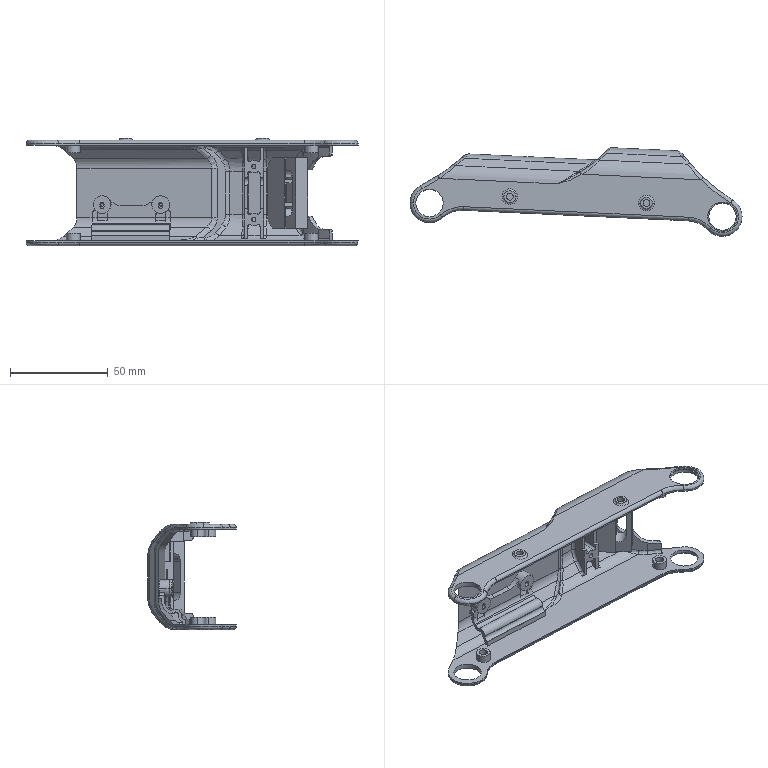Part | NX | features BREP 3 | 3 solids | 391 faces | box 169.834 x 45.304 x 55 mm | volume 40622 mm3 | cylinder 157 | plane 136 | spline 76 | torus 22 | commonest cylinder face diameters 20 x20 2 x15 5 x10 7 x10 1.6 x8 2.2 x8